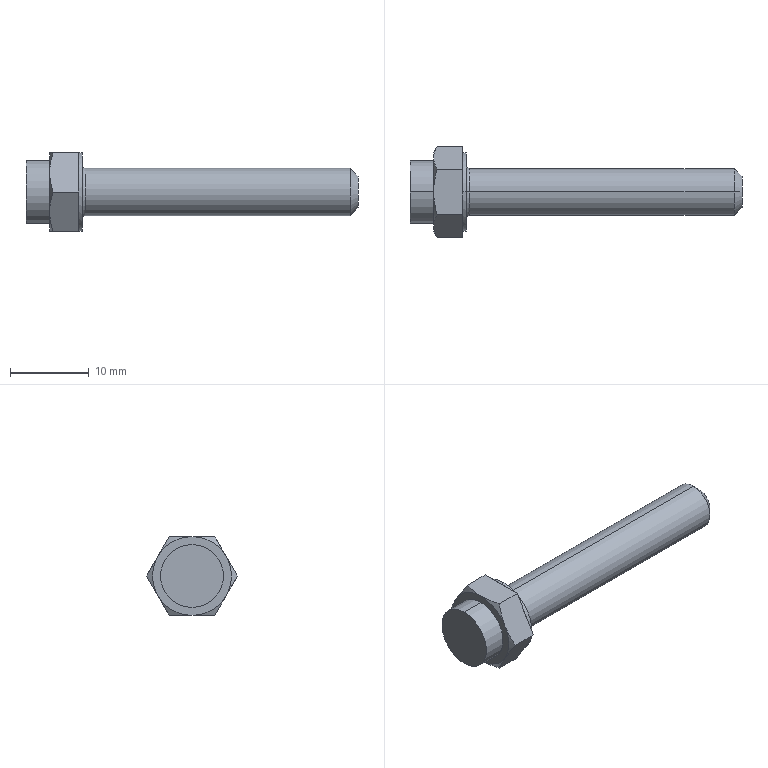Part | SolidWorks | features RevCut 4, ICE 2, Chamfer 1, Extrusion 1, Fillet 1, LPattern 1, Revolution 1 | 2 solids | 36 faces | box 42.15 x 11.547 x 10 mm | volume 1487 mm3 | plane 18 | cylinder 8 | cone 8 | torus 2 | commonest cylinder face diameters 8 x4 6 x2 10 x2
STEP:
#1=CARTESIAN_POINT('',(3.,0.,-4.));
#2=VERTEX_POINT('',#1);
#3=CARTESIAN_POINT('',(3.,0.,4.));
#4=VERTEX_POINT('',#3);
#5=CARTESIAN_POINT('',(3.,0.,0.));
#6=DIRECTION('',(-1.,0.,0.));
#7=DIRECTION('',(0.,0.,1.));
#8=AXIS2_PLACEMENT_3D('',#5,#6,#7);
#9=CIRCLE('',#8,4.);
#10=EDGE_CURVE('',#2,#4,#9,.T.);
#11=ORIENTED_EDGE('',*,*,#10,.F.);
#12=CARTESIAN_POINT('',(0.,0.,-4.));
#13=VERTEX_POINT('',#12);
#14=CARTESIAN_POINT('',(3.,0.,-4.));
#15=DIRECTION('',(-1.,0.,0.));
#16=VECTOR('',#15,1000.);
#17=LINE('',#14,#16);
#18=EDGE_CURVE('',#2,#13,#17,.T.);
#19=ORIENTED_EDGE('',*,*,#18,.T.);
#20=CARTESIAN_POINT('',(0.,0.,4.));
#21=VERTEX_POINT('',#20);
#22=CARTESIAN_POINT('',(0.,0.,0.));
#23=DIRECTION('',(-1.,0.,0.));
#24=DIRECTION('',(0.,0.,1.));
#25=AXIS2_PLACEMENT_3D('',#22,#23,#24);
#26=CIRCLE('',#25,4.);
#27=EDGE_CURVE('',#13,#21,#26,.T.);
#28=ORIENTED_EDGE('',*,*,#27,.T.);
#29=CARTESIAN_POINT('',(3.,0.,4.));
#30=DIRECTION('',(-1.,0.,0.));
#31=VECTOR('',#30,1000.);
#32=LINE('',#29,#31);
#33=EDGE_CURVE('',#4,#21,#32,.T.);
#34=ORIENTED_EDGE('',*,*,#33,.F.);
#35=EDGE_LOOP('',(#11,#19,#28,#34));
#36=FACE_OUTER_BOUND('',#35,.T.);
#37=CARTESIAN_POINT('',(3.,0.,0.));
#38=DIRECTION('',(-1.,0.,0.));
#39=DIRECTION('',(0.,0.,1.));
#40=AXIS2_PLACEMENT_3D('',#37,#38,#39);
#41=CYLINDRICAL_SURFACE('',#40,4.);
#42=ADVANCED_FACE('',(#36),#41,.F.);
#43=CARTESIAN_POINT('',(4.55,0.,3.));
#44=VERTEX_POINT('',#43);
#45=CARTESIAN_POINT('',(4.55,0.,-3.));
#46=VERTEX_POINT('',#45);
#47=CARTESIAN_POINT('',(4.55,0.,0.));
#48=DIRECTION('',(1.,0.,0.));
#49=DIRECTION('',(0.,0.,-1.));
#50=AXIS2_PLACEMENT_3D('',#47,#48,#49);
#51=CIRCLE('',#50,3.);
#52=EDGE_CURVE('',#44,#46,#51,.T.);
#53=ORIENTED_EDGE('',*,*,#52,.F.);
#54=CARTESIAN_POINT('',(4.15,0.,3.4));
#55=VERTEX_POINT('',#54);
#56=CARTESIAN_POINT('',(4.55,0.,3.4));
#57=DIRECTION('',(0.,1.,0.));
#58=DIRECTION('',(0.,0.,1.));
#59=AXIS2_PLACEMENT_3D('',#56,#57,#58);
#60=CIRCLE('',#59,0.4);
#61=EDGE_CURVE('',#44,#55,#60,.T.);
#62=ORIENTED_EDGE('',*,*,#61,.T.);
#63=CARTESIAN_POINT('',(4.15,0.,-3.4));
#64=VERTEX_POINT('',#63);
#65=CARTESIAN_POINT('',(4.15,0.,0.));
#66=DIRECTION('',(-1.,0.,0.));
#67=DIRECTION('',(0.,0.,-1.));
#68=AXIS2_PLACEMENT_3D('',#65,#66,#67);
#69=CIRCLE('',#68,3.4);
#70=EDGE_CURVE('',#64,#55,#69,.T.);
#71=ORIENTED_EDGE('',*,*,#70,.F.);
#72=CARTESIAN_POINT('',(4.55,0.,-3.4));
#73=DIRECTION('',(0.,-1.,0.));
#74=DIRECTION('',(0.,0.,-1.));
#75=AXIS2_PLACEMENT_3D('',#72,#73,#74);
#76=CIRCLE('',#75,0.4);
#77=EDGE_CURVE('',#46,#64,#76,.T.);
#78=ORIENTED_EDGE('',*,*,#77,.F.);
#79=EDGE_LOOP('',(#53,#62,#71,#78));
#80=FACE_OUTER_BOUND('',#79,.T.);
#81=CARTESIAN_POINT('',(4.55,0.,0.));
#82=DIRECTION('',(1.,0.,0.));
#83=DIRECTION('',(0.,0.,-1.));
#84=AXIS2_PLACEMENT_3D('',#81,#82,#83);
#85=TOROIDAL_SURFACE('',#84,3.4,0.4);
#86=ADVANCED_FACE('',(#80),#85,.F.);
#87=CARTESIAN_POINT('',(39.15,0.,-2.));
#88=VERTEX_POINT('',#87);
#89=CARTESIAN_POINT('',(39.15,0.,2.));
#90=VERTEX_POINT('',#89);
#91=CARTESIAN_POINT('',(39.15,0.,0.));
#92=DIRECTION('',(1.,0.,0.));
#93=DIRECTION('',(0.,0.,1.));
#94=AXIS2_PLACEMENT_3D('',#91,#92,#93);
#95=CIRCLE('',#94,2.);
#96=EDGE_CURVE('',#88,#90,#95,.T.);
#97=ORIENTED_EDGE('',*,*,#96,.F.);
#98=CARTESIAN_POINT('',(38.15,0.,-3.));
#99=VERTEX_POINT('',#98);
#100=CARTESIAN_POINT('',(38.15,0.,-3.));
#101=DIRECTION('',(-0.7071,0.,-0.7071));
#102=VECTOR('',#101,1000.);
#103=LINE('',#100,#102);
#104=EDGE_CURVE('',#88,#99,#103,.T.);
#105=ORIENTED_EDGE('',*,*,#104,.T.);
#106=CARTESIAN_POINT('',(38.15,0.,3.));
#107=VERTEX_POINT('',#106);
#108=CARTESIAN_POINT('',(38.15,0.,0.));
#109=DIRECTION('',(-1.,0.,0.));
#110=DIRECTION('',(0.,0.,1.));
#111=AXIS2_PLACEMENT_3D('',#108,#109,#110);
#112=CIRCLE('',#111,3.);
#113=EDGE_CURVE('',#107,#99,#112,.T.);
#114=ORIENTED_EDGE('',*,*,#113,.F.);
#115=CARTESIAN_POINT('',(38.15,0.,3.));
#116=DIRECTION('',(-0.7071,0.,0.7071));
#117=VECTOR('',#116,1000.);
#118=LINE('',#115,#117);
#119=EDGE_CURVE('',#90,#107,#118,.T.);
#120=ORIENTED_EDGE('',*,*,#119,.F.);
#121=EDGE_LOOP('',(#97,#105,#114,#120));
#122=FACE_OUTER_BOUND('',#121,.T.);
#123=CARTESIAN_POINT('',(38.15,0.,0.));
#124=DIRECTION('',(-1.,0.,0.));
#125=DIRECTION('',(0.,0.,1.));
#126=AXIS2_PLACEMENT_3D('',#123,#124,#125);
#127=CONICAL_SURFACE('',#126,3.,0.7854);
#128=ADVANCED_FACE('',(#122),#127,.T.);
#129=ORIENTED_EDGE('',*,*,#113,.T.);
#130=CARTESIAN_POINT('',(0.,0.,-3.));
#131=DIRECTION('',(-1.,0.,0.));
#132=VECTOR('',#131,1000.);
#133=LINE('',#130,#132);
#134=EDGE_CURVE('',#99,#46,#133,.T.);
#135=ORIENTED_EDGE('',*,*,#134,.T.);
#136=CARTESIAN_POINT('',(4.55,0.,0.));
#137=DIRECTION('',(1.,0.,0.));
#138=DIRECTION('',(0.,0.,-1.));
#139=AXIS2_PLACEMENT_3D('',#136,#137,#138);
#140=CIRCLE('',#139,3.);
#141=EDGE_CURVE('',#46,#44,#140,.T.);
#142=ORIENTED_EDGE('',*,*,#141,.T.);
#143=CARTESIAN_POINT('',(0.,0.,3.));
#144=DIRECTION('',(-1.,0.,0.));
#145=VECTOR('',#144,1000.);
#146=LINE('',#143,#145);
#147=EDGE_CURVE('',#107,#44,#146,.T.);
#148=ORIENTED_EDGE('',*,*,#147,.F.);
#149=EDGE_LOOP('',(#129,#135,#142,#148));
#150=FACE_OUTER_BOUND('',#149,.T.);
#151=CARTESIAN_POINT('',(0.,0.,0.));
#152=DIRECTION('',(-1.,0.,0.));
#153=DIRECTION('',(0.,0.,1.));
#154=AXIS2_PLACEMENT_3D('',#151,#152,#153);
#155=CYLINDRICAL_SURFACE('',#154,3.);
#156=ADVANCED_FACE('',(#150),#155,.T.);
#157=CARTESIAN_POINT('',(4.15,0.,-5.));
#158=VERTEX_POINT('',#157);
#159=CARTESIAN_POINT('',(4.15,0.,5.));
#160=VERTEX_POINT('',#159);
#161=CARTESIAN_POINT('',(4.15,0.,0.));
#162=DIRECTION('',(1.,0.,0.));
#163=DIRECTION('',(0.,0.,-1.));
#164=AXIS2_PLACEMENT_3D('',#161,#162,#163);
#165=CIRCLE('',#164,5.);
#166=EDGE_CURVE('',#158,#160,#165,.T.);
#167=ORIENTED_EDGE('',*,*,#166,.F.);
#168=CARTESIAN_POINT('',(3.65,0.,-5.));
#169=VERTEX_POINT('',#168);
#170=CARTESIAN_POINT('',(0.,0.,-5.));
#171=DIRECTION('',(-1.,0.,0.));
#172=VECTOR('',#171,1000.);
#173=LINE('',#170,#172);
#174=EDGE_CURVE('',#158,#169,#173,.T.);
#175=ORIENTED_EDGE('',*,*,#174,.T.);
#176=CARTESIAN_POINT('',(3.65,4.33,-2.5));
#177=VERTEX_POINT('',#176);
#178=CARTESIAN_POINT('',(3.65,0.,0.));
#179=DIRECTION('',(-1.,0.,0.));
#180=DIRECTION('',(0.,0.,1.));
#181=AXIS2_PLACEMENT_3D('',#178,#179,#180);
#182=CIRCLE('',#181,5.);
#183=EDGE_CURVE('',#177,#169,#182,.T.);
#184=ORIENTED_EDGE('',*,*,#183,.F.);
#185=CARTESIAN_POINT('',(3.65,4.33,2.5));
#186=VERTEX_POINT('',#185);
#187=CARTESIAN_POINT('',(3.65,0.,0.));
#188=DIRECTION('',(-1.,0.,0.));
#189=DIRECTION('',(0.,0.,1.));
#190=AXIS2_PLACEMENT_3D('',#187,#188,#189);
#191=CIRCLE('',#190,5.);
#192=EDGE_CURVE('',#186,#177,#191,.T.);
#193=ORIENTED_EDGE('',*,*,#192,.F.);
#194=CARTESIAN_POINT('',(3.65,0.,5.));
#195=VERTEX_POINT('',#194);
#196=CARTESIAN_POINT('',(3.65,0.,0.));
#197=DIRECTION('',(-1.,0.,0.));
#198=DIRECTION('',(0.,0.,1.));
#199=AXIS2_PLACEMENT_3D('',#196,#197,#198);
#200=CIRCLE('',#199,5.);
#201=EDGE_CURVE('',#195,#186,#200,.T.);
#202=ORIENTED_EDGE('',*,*,#201,.F.);
#203=CARTESIAN_POINT('',(0.,0.,5.));
#204=DIRECTION('',(-1.,0.,0.));
#205=VECTOR('',#204,1000.);
#206=LINE('',#203,#205);
#207=EDGE_CURVE('',#160,#195,#206,.T.);
#208=ORIENTED_EDGE('',*,*,#207,.F.);
#209=EDGE_LOOP('',(#167,#175,#184,#193,#202,#208));
#210=FACE_OUTER_BOUND('',#209,.T.);
#211=CARTESIAN_POINT('',(0.,0.,0.));
#212=DIRECTION('',(-1.,0.,0.));
#213=DIRECTION('',(0.,0.,1.));
#214=AXIS2_PLACEMENT_3D('',#211,#212,#213);
#215=CYLINDRICAL_SURFACE('',#214,5.);
#216=ADVANCED_FACE('',(#210),#215,.T.);
#217=CARTESIAN_POINT('',(3.65,2.887,-5.));
#218=VERTEX_POINT('',#217);
#219=CARTESIAN_POINT('',(3.65,2.887,-5.));
#220=DIRECTION('',(0.,0.5,0.866));
#221=VECTOR('',#220,1000.);
#222=LINE('',#219,#221);
#223=EDGE_CURVE('',#218,#177,#222,.T.);
#224=ORIENTED_EDGE('',*,*,#223,.F.);
#225=CARTESIAN_POINT('',(0.4466,2.887,-5.));
#226=VERTEX_POINT('',#225);
#227=CARTESIAN_POINT('',(4.15,2.887,-5.));
#228=DIRECTION('',(-1.,0.,0.));
#229=VECTOR('',#228,1000.);
#230=LINE('',#227,#229);
#231=EDGE_CURVE('',#218,#226,#230,.T.);
#232=ORIENTED_EDGE('',*,*,#231,.T.);
#233=CARTESIAN_POINT('',(0.,4.33,-2.5));
#234=VERTEX_POINT('',#233);
#235=CARTESIAN_POINT('',(0.,4.33,-2.5));
#236=CARTESIAN_POINT('',(0.,4.208,-2.712));
#237=CARTESIAN_POINT('',(0.01056,4.085,-2.925));
#238=CARTESIAN_POINT('',(0.0514,3.841,-3.347));
#239=CARTESIAN_POINT('',(0.08166,3.72,-3.556));
#240=CARTESIAN_POINT('',(0.1983,3.36,-4.181));
#241=CARTESIAN_POINT('',(0.3106,3.122,-4.592));
#242=CARTESIAN_POINT('',(0.4466,2.887,-5.));
#243=B_SPLINE_CURVE_WITH_KNOTS('',3,(#235,#236,#237,#238,#239,#240,#241,#242),.UNSPECIFIED.,.F.,.F.,(4,2,2,4),(0.002921,0.003649,0.004376,0.005831),.UNSPECIFIED.);
#244=EDGE_CURVE('',#234,#226,#243,.T.);
#245=ORIENTED_EDGE('',*,*,#244,.F.);
#246=CARTESIAN_POINT('',(0.4466,5.774,0.));
#247=VERTEX_POINT('',#246);
#248=CARTESIAN_POINT('',(0.4466,5.774,0.));
#249=CARTESIAN_POINT('',(0.1739,5.301,-0.8179));
#250=CARTESIAN_POINT('',(0.,4.822,-1.648));
#251=CARTESIAN_POINT('',(0.,4.33,-2.5));
#252=B_SPLINE_CURVE_WITH_KNOTS('',3,(#248,#249,#250,#251),.UNSPECIFIED.,.F.,.F.,(4,4),(0.000000238,0.002921),.UNSPECIFIED.);
#253=EDGE_CURVE('',#247,#234,#252,.T.);
#254=ORIENTED_EDGE('',*,*,#253,.F.);
#255=CARTESIAN_POINT('',(3.65,5.774,0.));
#256=VERTEX_POINT('',#255);
#257=CARTESIAN_POINT('',(4.15,5.774,0.));
#258=DIRECTION('',(-1.,0.,0.));
#259=VECTOR('',#258,1000.);
#260=LINE('',#257,#259);
#261=EDGE_CURVE('',#256,#247,#260,.T.);
#262=ORIENTED_EDGE('',*,*,#261,.F.);
#263=CARTESIAN_POINT('',(3.65,2.887,-5.));
#264=DIRECTION('',(0.,0.5,0.866));
#265=VECTOR('',#264,1000.);
#266=LINE('',#263,#265);
#267=EDGE_CURVE('',#177,#256,#266,.T.);
#268=ORIENTED_EDGE('',*,*,#267,.F.);
#269=EDGE_LOOP('',(#224,#232,#245,#254,#262,#268));
#270=FACE_OUTER_BOUND('',#269,.T.);
#271=CARTESIAN_POINT('',(4.15,2.887,-5.));
#272=DIRECTION('',(0.,-0.866,0.5));
#273=DIRECTION('',(0.,-0.5,-0.866));
#274=AXIS2_PLACEMENT_3D('',#271,#272,#273);
#275=PLANE('',#274);
#276=ADVANCED_FACE('',(#270),#275,.F.);
#277=CARTESIAN_POINT('',(3.65,5.774,0.));
#278=DIRECTION('',(0.,-0.5,0.866));
#279=VECTOR('',#278,1000.);
#280=LINE('',#277,#279);
#281=EDGE_CURVE('',#256,#186,#280,.T.);
#282=ORIENTED_EDGE('',*,*,#281,.F.);
#283=ORIENTED_EDGE('',*,*,#261,.T.);
#284=CARTESIAN_POINT('',(0.,4.33,2.5));
#285=VERTEX_POINT('',#284);
#286=CARTESIAN_POINT('',(0.,4.33,2.5));
#287=CARTESIAN_POINT('',(0.,4.453,2.288));
#288=CARTESIAN_POINT('',(0.01056,4.576,2.075));
#289=CARTESIAN_POINT('',(0.0514,4.819,1.653));
#290=CARTESIAN_POINT('',(0.08166,4.94,1.444));
#291=CARTESIAN_POINT('',(0.1983,5.3,0.8193));
#292=CARTESIAN_POINT('',(0.3106,5.538,0.4079));
#293=CARTESIAN_POINT('',(0.4466,5.774,0.));
#294=B_SPLINE_CURVE_WITH_KNOTS('',3,(#286,#287,#288,#289,#290,#291,#292,#293),.UNSPECIFIED.,.F.,.F.,(4,2,2,4),(0.002921,0.003649,0.004376,0.005831),.UNSPECIFIED.);
#295=EDGE_CURVE('',#285,#247,#294,.T.);
#296=ORIENTED_EDGE('',*,*,#295,.F.);
#297=CARTESIAN_POINT('',(0.4466,2.887,5.));
#298=VERTEX_POINT('',#297);
#299=CARTESIAN_POINT('',(0.4466,2.887,5.));
#300=CARTESIAN_POINT('',(0.1739,3.359,4.182));
#301=CARTESIAN_POINT('',(0.,3.838,3.352));
#302=CARTESIAN_POINT('',(0.,4.33,2.5));
#303=B_SPLINE_CURVE_WITH_KNOTS('',3,(#299,#300,#301,#302),.UNSPECIFIED.,.F.,.F.,(4,4),(0.000000238,0.002921),.UNSPECIFIED.);
#304=EDGE_CURVE('',#298,#285,#303,.T.);
#305=ORIENTED_EDGE('',*,*,#304,.F.);
#306=CARTESIAN_POINT('',(3.65,2.887,5.));
#307=VERTEX_POINT('',#306);
#308=CARTESIAN_POINT('',(4.15,2.887,5.));
#309=DIRECTION('',(-1.,0.,0.));
#310=VECTOR('',#309,1000.);
#311=LINE('',#308,#310);
#312=EDGE_CURVE('',#307,#298,#311,.T.);
#313=ORIENTED_EDGE('',*,*,#312,.F.);
#314=CARTESIAN_POINT('',(3.65,5.774,0.));
#315=DIRECTION('',(0.,-0.5,0.866));
#316=VECTOR('',#315,1000.);
#317=LINE('',#314,#316);
#318=EDGE_CURVE('',#186,#307,#317,.T.);
#319=ORIENTED_EDGE('',*,*,#318,.F.);
#320=EDGE_LOOP('',(#282,#283,#296,#305,#313,#319));
#321=FACE_OUTER_BOUND('',#320,.T.);
#322=CARTESIAN_POINT('',(4.15,5.774,0.));
#323=DIRECTION('',(0.,-0.866,-0.5));
#324=DIRECTION('',(0.,0.5,-0.866));
#325=AXIS2_PLACEMENT_3D('',#322,#323,#324);
#326=PLANE('',#325);
#327=ADVANCED_FACE('',(#321),#326,.F.);
#328=CARTESIAN_POINT('',(3.65,2.887,5.));
#329=DIRECTION('',(0.,-1.,0.));
#330=VECTOR('',#329,1000.);
#331=LINE('',#328,#330);
#332=EDGE_CURVE('',#307,#195,#331,.T.);
#333=ORIENTED_EDGE('',*,*,#332,.F.);
#334=ORIENTED_EDGE('',*,*,#312,.T.);
#335=CARTESIAN_POINT('',(0.,0.,5.));
#336=VERTEX_POINT('',#335);
#337=CARTESIAN_POINT('',(0.,0.,5.));
#338=CARTESIAN_POINT('',(0.,0.4887,5.));
#339=CARTESIAN_POINT('',(0.04321,0.9837,5.));
#340=CARTESIAN_POINT('',(0.1996,1.947,5.));
#341=CARTESIAN_POINT('',(0.3118,2.42,5.));
#342=CARTESIAN_POINT('',(0.4466,2.887,5.));
#343=B_SPLINE_CURVE_WITH_KNOTS('',3,(#337,#338,#339,#340,#341,#342),.UNSPECIFIED.,.F.,.F.,(4,2,4),(0.008262,0.009724,0.01119),.UNSPECIFIED.);
#344=EDGE_CURVE('',#336,#298,#343,.T.);
#345=ORIENTED_EDGE('',*,*,#344,.F.);
#346=CARTESIAN_POINT('',(0.4466,-2.887,5.));
#347=VERTEX_POINT('',#346);
#348=CARTESIAN_POINT('',(0.4466,-2.887,5.));
#349=CARTESIAN_POINT('',(0.3109,-2.417,5.));
#350=CARTESIAN_POINT('',(0.1973,-1.936,5.));
#351=CARTESIAN_POINT('',(0.04202,-0.9731,5.));
#352=CARTESIAN_POINT('',(0.,-0.4884,5.));
#353=CARTESIAN_POINT('',(0.,0.,5.));
#354=B_SPLINE_CURVE_WITH_KNOTS('',3,(#348,#349,#350,#351,#352,#353),.UNSPECIFIED.,.F.,.F.,(4,2,4),(0.00534,0.006801,0.008262),.UNSPECIFIED.);
#355=EDGE_CURVE('',#347,#336,#354,.T.);
#356=ORIENTED_EDGE('',*,*,#355,.F.);
#357=CARTESIAN_POINT('',(3.65,-2.887,5.));
#358=VERTEX_POINT('',#357);
#359=CARTESIAN_POINT('',(4.15,-2.887,5.));
#360=DIRECTION('',(-1.,0.,0.));
#361=VECTOR('',#360,1000.);
#362=LINE('',#359,#361);
#363=EDGE_CURVE('',#358,#347,#362,.T.);
#364=ORIENTED_EDGE('',*,*,#363,.F.);
#365=CARTESIAN_POINT('',(3.65,2.887,5.));
#366=DIRECTION('',(0.,-1.,0.));
#367=VECTOR('',#366,1000.);
#368=LINE('',#365,#367);
#369=EDGE_CURVE('',#195,#358,#368,.T.);
#370=ORIENTED_EDGE('',*,*,#369,.F.);
#371=EDGE_LOOP('',(#333,#334,#345,#356,#364,#370));
#372=FACE_OUTER_BOUND('',#371,.T.);
#373=CARTESIAN_POINT('',(4.15,2.887,5.));
#374=DIRECTION('',(0.,0.,-1.));
#375=DIRECTION('',(-1.,0.,0.));
#376=AXIS2_PLACEMENT_3D('',#373,#374,#375);
#377=PLANE('',#376);
#378=ADVANCED_FACE('',(#372),#377,.F.);
#379=CARTESIAN_POINT('',(3.65,-4.33,2.5));
#380=VERTEX_POINT('',#379);
#381=CARTESIAN_POINT('',(3.65,-5.774,0.));
#382=DIRECTION('',(0.,-0.5,-0.866));
#383=VECTOR('',#382,1000.);
#384=LINE('',#381,#383);
#385=EDGE_CURVE('',#358,#380,#384,.T.);
#386=ORIENTED_EDGE('',*,*,#385,.F.);
#387=ORIENTED_EDGE('',*,*,#363,.T.);
#388=CARTESIAN_POINT('',(0.,-4.33,2.5));
#389=VERTEX_POINT('',#388);
#390=CARTESIAN_POINT('',(0.,-4.33,2.5));
#391=CARTESIAN_POINT('',(0.,-4.208,2.712));
#392=CARTESIAN_POINT('',(0.01056,-4.085,2.925));
#393=CARTESIAN_POINT('',(0.0514,-3.841,3.347));
#394=CARTESIAN_POINT('',(0.08166,-3.72,3.556));
#395=CARTESIAN_POINT('',(0.1983,-3.36,4.181));
#396=CARTESIAN_POINT('',(0.3106,-3.122,4.592));
#397=CARTESIAN_POINT('',(0.4466,-2.887,5.));
#398=B_SPLINE_CURVE_WITH_KNOTS('',3,(#390,#391,#392,#393,#394,#395,#396,#397),.UNSPECIFIED.,.F.,.F.,(4,2,2,4),(0.002921,0.003649,0.004376,0.005831),.UNSPECIFIED.);
#399=EDGE_CURVE('',#389,#347,#398,.T.);
#400=ORIENTED_EDGE('',*,*,#399,.F.);
#401=CARTESIAN_POINT('',(0.4466,-5.774,0.));
#402=VERTEX_POINT('',#401);
#403=CARTESIAN_POINT('',(0.4466,-5.774,0.));
#404=CARTESIAN_POINT('',(0.1739,-5.301,0.8179));
#405=CARTESIAN_POINT('',(0.,-4.822,1.648));
#406=CARTESIAN_POINT('',(0.,-4.33,2.5));
#407=B_SPLINE_CURVE_WITH_KNOTS('',3,(#403,#404,#405,#406),.UNSPECIFIED.,.F.,.F.,(4,4),(0.000000238,0.002921),.UNSPECIFIED.);
#408=EDGE_CURVE('',#402,#389,#407,.T.);
#409=ORIENTED_EDGE('',*,*,#408,.F.);
#410=CARTESIAN_POINT('',(3.65,-5.774,0.));
#411=VERTEX_POINT('',#410);
#412=CARTESIAN_POINT('',(4.15,-5.774,0.));
#413=DIRECTION('',(-1.,0.,0.));
#414=VECTOR('',#413,1000.);
#415=LINE('',#412,#414);
#416=EDGE_CURVE('',#411,#402,#415,.T.);
#417=ORIENTED_EDGE('',*,*,#416,.F.);
#418=CARTESIAN_POINT('',(3.65,-5.774,0.));
#419=DIRECTION('',(0.,-0.5,-0.866));
#420=VECTOR('',#419,1000.);
#421=LINE('',#418,#420);
#422=EDGE_CURVE('',#380,#411,#421,.T.);
#423=ORIENTED_EDGE('',*,*,#422,.F.);
#424=EDGE_LOOP('',(#386,#387,#400,#409,#417,#423));
#425=FACE_OUTER_BOUND('',#424,.T.);
#426=CARTESIAN_POINT('',(4.15,-5.774,0.));
#427=DIRECTION('',(0.,0.866,-0.5));
#428=DIRECTION('',(0.,0.5,0.866));
#429=AXIS2_PLACEMENT_3D('',#426,#427,#428);
#430=PLANE('',#429);
#431=ADVANCED_FACE('',(#425),#430,.F.);
#432=CARTESIAN_POINT('',(3.65,-4.33,-2.5));
#433=VERTEX_POINT('',#432);
#434=CARTESIAN_POINT('',(3.65,-2.887,-5.));
#435=DIRECTION('',(0.,0.5,-0.866));
#436=VECTOR('',#435,1000.);
#437=LINE('',#434,#436);
#438=EDGE_CURVE('',#411,#433,#437,.T.);
#439=ORIENTED_EDGE('',*,*,#438,.F.);
#440=ORIENTED_EDGE('',*,*,#416,.T.);
#441=CARTESIAN_POINT('',(0.,-4.33,-2.5));
#442=VERTEX_POINT('',#441);
#443=CARTESIAN_POINT('',(0.,-4.33,-2.5));
#444=CARTESIAN_POINT('',(0.,-4.453,-2.288));
#445=CARTESIAN_POINT('',(0.01056,-4.576,-2.075));
#446=CARTESIAN_POINT('',(0.0514,-4.819,-1.653));
#447=CARTESIAN_POINT('',(0.08166,-4.94,-1.444));
#448=CARTESIAN_POINT('',(0.1983,-5.3,-0.8193));
#449=CARTESIAN_POINT('',(0.3106,-5.538,-0.4079));
#450=CARTESIAN_POINT('',(0.4466,-5.774,0.));
#451=B_SPLINE_CURVE_WITH_KNOTS('',3,(#443,#444,#445,#446,#447,#448,#449,#450),.UNSPECIFIED.,.F.,.F.,(4,2,2,4),(0.002921,0.003649,0.004376,0.005831),.UNSPECIFIED.);
#452=EDGE_CURVE('',#442,#402,#451,.T.);
#453=ORIENTED_EDGE('',*,*,#452,.F.);
#454=CARTESIAN_POINT('',(0.4466,-2.887,-5.));
#455=VERTEX_POINT('',#454);
#456=CARTESIAN_POINT('',(0.4466,-2.887,-5.));
#457=CARTESIAN_POINT('',(0.1739,-3.359,-4.182));
#458=CARTESIAN_POINT('',(0.,-3.838,-3.352));
#459=CARTESIAN_POINT('',(0.,-4.33,-2.5));
#460=B_SPLINE_CURVE_WITH_KNOTS('',3,(#456,#457,#458,#459),.UNSPECIFIED.,.F.,.F.,(4,4),(0.000000238,0.002921),.UNSPECIFIED.);
#461=EDGE_CURVE('',#455,#442,#460,.T.);
#462=ORIENTED_EDGE('',*,*,#461,.F.);
#463=CARTESIAN_POINT('',(3.65,-2.887,-5.));
#464=VERTEX_POINT('',#463);
#465=CARTESIAN_POINT('',(4.15,-2.887,-5.));
#466=DIRECTION('',(-1.,0.,0.));
#467=VECTOR('',#466,1000.);
#468=LINE('',#465,#467);
#469=EDGE_CURVE('',#464,#455,#468,.T.);
#470=ORIENTED_EDGE('',*,*,#469,.F.);
#471=CARTESIAN_POINT('',(3.65,-2.887,-5.));
#472=DIRECTION('',(0.,0.5,-0.866));
#473=VECTOR('',#472,1000.);
#474=LINE('',#471,#473);
#475=EDGE_CURVE('',#433,#464,#474,.T.);
#476=ORIENTED_EDGE('',*,*,#475,.F.);
#477=EDGE_LOOP('',(#439,#440,#453,#462,#470,#476));
#478=FACE_OUTER_BOUND('',#477,.T.);
#479=CARTESIAN_POINT('',(4.15,-2.887,-5.));
#480=DIRECTION('',(0.,0.866,0.5));
#481=DIRECTION('',(0.,-0.5,0.866));
#482=AXIS2_PLACEMENT_3D('',#479,#480,#481);
#483=PLANE('',#482);
#484=ADVANCED_FACE('',(#478),#483,.F.);
#485=CARTESIAN_POINT('',(3.65,2.887,-5.));
#486=DIRECTION('',(0.,1.,0.));
#487=VECTOR('',#486,1000.);
#488=LINE('',#485,#487);
#489=EDGE_CURVE('',#464,#169,#488,.T.);
#490=ORIENTED_EDGE('',*,*,#489,.F.);
#491=ORIENTED_EDGE('',*,*,#469,.T.);
#492=CARTESIAN_POINT('',(0.,0.,-5.));
#493=VERTEX_POINT('',#492);
#494=CARTESIAN_POINT('',(0.,0.,-5.));
#495=CARTESIAN_POINT('',(0.,-0.4884,-5.));
#496=CARTESIAN_POINT('',(0.04202,-0.9731,-5.));
#497=CARTESIAN_POINT('',(0.1973,-1.936,-5.));
#498=CARTESIAN_POINT('',(0.3109,-2.417,-5.));
#499=CARTESIAN_POINT('',(0.4466,-2.887,-5.));
#500=B_SPLINE_CURVE_WITH_KNOTS('',3,(#494,#495,#496,#497,#498,#499),.UNSPECIFIED.,.F.,.F.,(4,2,4),(0.01799,0.01945,0.02091),.UNSPECIFIED.);
#501=EDGE_CURVE('',#493,#455,#500,.T.);
#502=ORIENTED_EDGE('',*,*,#501,.F.);
#503=CARTESIAN_POINT('',(0.4466,2.887,-5.));
#504=CARTESIAN_POINT('',(0.3118,2.42,-5.));
#505=CARTESIAN_POINT('',(0.1996,1.947,-5.));
#506=CARTESIAN_POINT('',(0.04321,0.9837,-5.));
#507=CARTESIAN_POINT('',(0.,0.4887,-5.));
#508=CARTESIAN_POINT('',(0.,0.,-5.));
#509=B_SPLINE_CURVE_WITH_KNOTS('',3,(#503,#504,#505,#506,#507,#508),.UNSPECIFIED.,.F.,.F.,(4,2,4),(0.01507,0.01653,0.01799),.UNSPECIFIED.);
#510=EDGE_CURVE('',#226,#493,#509,.T.);
#511=ORIENTED_EDGE('',*,*,#510,.F.);
#512=ORIENTED_EDGE('',*,*,#231,.F.);
#513=CARTESIAN_POINT('',(3.65,2.887,-5.));
#514=DIRECTION('',(0.,1.,0.));
#515=VECTOR('',#514,1000.);
#516=LINE('',#513,#515);
#517=EDGE_CURVE('',#169,#218,#516,.T.);
#518=ORIENTED_EDGE('',*,*,#517,.F.);
#519=EDGE_LOOP('',(#490,#491,#502,#511,#512,#518));
#520=FACE_OUTER_BOUND('',#519,.T.);
#521=CARTESIAN_POINT('',(4.15,2.887,-5.));
#522=DIRECTION('',(0.,0.,1.));
#523=DIRECTION('',(1.,0.,0.));
#524=AXIS2_PLACEMENT_3D('',#521,#522,#523);
#525=PLANE('',#524);
#526=ADVANCED_FACE('',(#520),#525,.F.);
#527=ORIENTED_EDGE('',*,*,#461,.T.);
#528=CARTESIAN_POINT('',(0.,0.,0.));
#529=DIRECTION('',(1.,0.,0.));
#530=DIRECTION('',(0.,0.,-1.));
#531=AXIS2_PLACEMENT_3D('',#528,#529,#530);
#532=CIRCLE('',#531,5.);
#533=EDGE_CURVE('',#442,#493,#532,.T.);
#534=ORIENTED_EDGE('',*,*,#533,.T.);
#535=ORIENTED_EDGE('',*,*,#501,.T.);
#536=EDGE_LOOP('',(#527,#534,#535));
#537=FACE_OUTER_BOUND('',#536,.T.);
#538=CARTESIAN_POINT('',(0.,0.,0.));
#539=DIRECTION('',(1.,0.,0.));
#540=DIRECTION('',(0.,0.,-1.));
#541=AXIS2_PLACEMENT_3D('',#538,#539,#540);
#542=CONICAL_SURFACE('',#541,5.,1.047);
#543=ADVANCED_FACE('',(#537),#542,.T.);
#544=ORIENTED_EDGE('',*,*,#408,.T.);
#545=CARTESIAN_POINT('',(0.,0.,0.));
#546=DIRECTION('',(1.,0.,0.));
#547=DIRECTION('',(0.,0.,-1.));
#548=AXIS2_PLACEMENT_3D('',#545,#546,#547);
#549=CIRCLE('',#548,5.);
#550=EDGE_CURVE('',#389,#442,#549,.T.);
#551=ORIENTED_EDGE('',*,*,#550,.T.);
#552=ORIENTED_EDGE('',*,*,#452,.T.);
#553=EDGE_LOOP('',(#544,#551,#552));
#554=FACE_OUTER_BOUND('',#553,.T.);
#555=CARTESIAN_POINT('',(0.,0.,0.));
#556=DIRECTION('',(1.,0.,0.));
#557=DIRECTION('',(0.,0.,-1.));
#558=AXIS2_PLACEMENT_3D('',#555,#556,#557);
#559=CONICAL_SURFACE('',#558,5.,1.047);
#560=ADVANCED_FACE('',(#554),#559,.T.);
#561=ORIENTED_EDGE('',*,*,#355,.T.);
#562=CARTESIAN_POINT('',(0.,0.,0.));
#563=DIRECTION('',(1.,0.,0.));
#564=DIRECTION('',(0.,0.,-1.));
#565=AXIS2_PLACEMENT_3D('',#562,#563,#564);
#566=CIRCLE('',#565,5.);
#567=EDGE_CURVE('',#336,#389,#566,.T.);
#568=ORIENTED_EDGE('',*,*,#567,.T.);
#569=ORIENTED_EDGE('',*,*,#399,.T.);
#570=EDGE_LOOP('',(#561,#568,#569));
#571=FACE_OUTER_BOUND('',#570,.T.);
#572=CARTESIAN_POINT('',(0.,0.,0.));
#573=DIRECTION('',(1.,0.,0.));
#574=DIRECTION('',(0.,0.,-1.));
#575=AXIS2_PLACEMENT_3D('',#572,#573,#574);
#576=CONICAL_SURFACE('',#575,5.,1.047);
#577=ADVANCED_FACE('',(#571),#576,.T.);
#578=ORIENTED_EDGE('',*,*,#344,.T.);
#579=ORIENTED_EDGE('',*,*,#304,.T.);
#580=CARTESIAN_POINT('',(0.,0.,0.));
#581=DIRECTION('',(-1.,0.,0.));
#582=DIRECTION('',(0.,0.,1.));
#583=AXIS2_PLACEMENT_3D('',#580,#581,#582);
#584=CIRCLE('',#583,5.);
#585=EDGE_CURVE('',#336,#285,#584,.T.);
#586=ORIENTED_EDGE('',*,*,#585,.F.);
#587=EDGE_LOOP('',(#578,#579,#586));
#588=FACE_OUTER_BOUND('',#587,.T.);
#589=CARTESIAN_POINT('',(0.,0.,0.));
#590=DIRECTION('',(1.,0.,0.));
#591=DIRECTION('',(0.,0.,-1.));
#592=AXIS2_PLACEMENT_3D('',#589,#590,#591);
#593=CONICAL_SURFACE('',#592,5.,1.047);
#594=ADVANCED_FACE('',(#588),#593,.T.);
#595=ORIENTED_EDGE('',*,*,#295,.T.);
#596=ORIENTED_EDGE('',*,*,#253,.T.);
#597=CARTESIAN_POINT('',(0.,0.,0.));
#598=DIRECTION('',(1.,0.,0.));
#599=DIRECTION('',(0.,0.,-1.));
#600=AXIS2_PLACEMENT_3D('',#597,#598,#599);
#601=CIRCLE('',#600,5.);
#602=EDGE_CURVE('',#234,#285,#601,.T.);
#603=ORIENTED_EDGE('',*,*,#602,.T.);
#604=EDGE_LOOP('',(#595,#596,#603));
#605=FACE_OUTER_BOUND('',#604,.T.);
#606=CARTESIAN_POINT('',(0.,0.,0.));
#607=DIRECTION('',(1.,0.,0.));
#608=DIRECTION('',(0.,0.,-1.));
#609=AXIS2_PLACEMENT_3D('',#606,#607,#608);
#610=CONICAL_SURFACE('',#609,5.,1.047);
#611=ADVANCED_FACE('',(#605),#610,.T.);
#612=ORIENTED_EDGE('',*,*,#244,.T.);
#613=ORIENTED_EDGE('',*,*,#510,.T.);
#614=CARTESIAN_POINT('',(0.,0.,0.));
#615=DIRECTION('',(1.,0.,0.));
#616=DIRECTION('',(0.,0.,-1.));
#617=AXIS2_PLACEMENT_3D('',#614,#615,#616);
#618=CIRCLE('',#617,5.);
#619=EDGE_CURVE('',#493,#234,#618,.T.);
#620=ORIENTED_EDGE('',*,*,#619,.T.);
#621=EDGE_LOOP('',(#612,#613,#620));
#622=FACE_OUTER_BOUND('',#621,.T.);
#623=CARTESIAN_POINT('',(0.,0.,0.));
#624=DIRECTION('',(1.,0.,0.));
#625=DIRECTION('',(0.,0.,-1.));
#626=AXIS2_PLACEMENT_3D('',#623,#624,#625);
#627=CONICAL_SURFACE('',#626,5.,1.047);
#628=ADVANCED_FACE('',(#622),#627,.T.);
#629=CARTESIAN_POINT('',(0.,0.,0.));
#630=DIRECTION('',(-1.,0.,0.));
#631=DIRECTION('',(0.,0.,1.));
#632=AXIS2_PLACEMENT_3D('',#629,#630,#631);
#633=CIRCLE('',#632,4.);
#634=EDGE_CURVE('',#21,#13,#633,.T.);
#635=ORIENTED_EDGE('',*,*,#634,.F.);
#636=ORIENTED_EDGE('',*,*,#27,.F.);
#637=EDGE_LOOP('',(#635,#636));
#638=FACE_BOUND('',#637,.T.);
#639=ORIENTED_EDGE('',*,*,#619,.F.);
#640=ORIENTED_EDGE('',*,*,#533,.F.);
#641=ORIENTED_EDGE('',*,*,#550,.F.);
#642=ORIENTED_EDGE('',*,*,#567,.F.);
#643=ORIENTED_EDGE('',*,*,#585,.T.);
#644=ORIENTED_EDGE('',*,*,#602,.F.);
#645=EDGE_LOOP('',(#639,#640,#641,#642,#643,#644));
#646=FACE_OUTER_BOUND('',#645,.T.);
#647=CARTESIAN_POINT('',(0.,5.774,0.));
#648=DIRECTION('',(1.,0.,0.));
#649=DIRECTION('',(0.,0.,-1.));
#650=AXIS2_PLACEMENT_3D('',#647,#648,#649);
#651=PLANE('',#650);
#652=ADVANCED_FACE('',(#638,#646),#651,.F.);
#653=ORIENTED_EDGE('',*,*,#223,.T.);
#654=ORIENTED_EDGE('',*,*,#183,.T.);
#655=ORIENTED_EDGE('',*,*,#517,.T.);
#656=EDGE_LOOP('',(#653,#654,#655));
#657=FACE_OUTER_BOUND('',#656,.T.);
#658=CARTESIAN_POINT('',(3.65,5.,0.));
#659=DIRECTION('',(1.,0.,0.));
#660=DIRECTION('',(0.,0.,-1.));
#661=AXIS2_PLACEMENT_3D('',#658,#659,#660);
#662=PLANE('',#661);
#663=ADVANCED_FACE('',(#657),#662,.T.);
#664=ORIENTED_EDGE('',*,*,#267,.T.);
#665=ORIENTED_EDGE('',*,*,#281,.T.);
#666=ORIENTED_EDGE('',*,*,#192,.T.);
#667=EDGE_LOOP('',(#664,#665,#666));
#668=FACE_OUTER_BOUND('',#667,.T.);
#669=CARTESIAN_POINT('',(3.65,5.,0.));
#670=DIRECTION('',(1.,0.,0.));
#671=DIRECTION('',(0.,0.,-1.));
#672=AXIS2_PLACEMENT_3D('',#669,#670,#671);
#673=PLANE('',#672);
#674=ADVANCED_FACE('',(#668),#673,.T.);
#675=ORIENTED_EDGE('',*,*,#318,.T.);
#676=ORIENTED_EDGE('',*,*,#332,.T.);
#677=ORIENTED_EDGE('',*,*,#201,.T.);
#678=EDGE_LOOP('',(#675,#676,#677));
#679=FACE_OUTER_BOUND('',#678,.T.);
#680=CARTESIAN_POINT('',(3.65,5.,0.));
#681=DIRECTION('',(1.,0.,0.));
#682=DIRECTION('',(0.,0.,-1.));
#683=AXIS2_PLACEMENT_3D('',#680,#681,#682);
#684=PLANE('',#683);
#685=ADVANCED_FACE('',(#679),#684,.T.);
#686=ORIENTED_EDGE('',*,*,#369,.T.);
#687=ORIENTED_EDGE('',*,*,#385,.T.);
#688=CARTESIAN_POINT('',(3.65,0.,0.));
#689=DIRECTION('',(-1.,0.,0.));
#690=DIRECTION('',(0.,0.,1.));
#691=AXIS2_PLACEMENT_3D('',#688,#689,#690);
#692=CIRCLE('',#691,5.);
#693=EDGE_CURVE('',#380,#195,#692,.T.);
#694=ORIENTED_EDGE('',*,*,#693,.T.);
#695=EDGE_LOOP('',(#686,#687,#694));
#696=FACE_OUTER_BOUND('',#695,.T.);
#697=CARTESIAN_POINT('',(3.65,5.,0.));
#698=DIRECTION('',(1.,0.,0.));
#699=DIRECTION('',(0.,0.,-1.));
#700=AXIS2_PLACEMENT_3D('',#697,#698,#699);
#701=PLANE('',#700);
#702=ADVANCED_FACE('',(#696),#701,.T.);
#703=ORIENTED_EDGE('',*,*,#422,.T.);
#704=ORIENTED_EDGE('',*,*,#438,.T.);
#705=CARTESIAN_POINT('',(3.65,0.,0.));
#706=DIRECTION('',(-1.,0.,0.));
#707=DIRECTION('',(0.,0.,1.));
#708=AXIS2_PLACEMENT_3D('',#705,#706,#707);
#709=CIRCLE('',#708,5.);
#710=EDGE_CURVE('',#433,#380,#709,.T.);
#711=ORIENTED_EDGE('',*,*,#710,.T.);
#712=EDGE_LOOP('',(#703,#704,#711));
#713=FACE_OUTER_BOUND('',#712,.T.);
#714=CARTESIAN_POINT('',(3.65,5.,0.));
#715=DIRECTION('',(1.,0.,0.));
#716=DIRECTION('',(0.,0.,-1.));
#717=AXIS2_PLACEMENT_3D('',#714,#715,#716);
#718=PLANE('',#717);
#719=ADVANCED_FACE('',(#713),#718,.T.);
#720=ORIENTED_EDGE('',*,*,#475,.T.);
#721=ORIENTED_EDGE('',*,*,#489,.T.);
#722=CARTESIAN_POINT('',(3.65,0.,0.));
#723=DIRECTION('',(-1.,0.,0.));
#724=DIRECTION('',(0.,0.,1.));
#725=AXIS2_PLACEMENT_3D('',#722,#723,#724);
#726=CIRCLE('',#725,5.);
#727=EDGE_CURVE('',#169,#433,#726,.T.);
#728=ORIENTED_EDGE('',*,*,#727,.T.);
#729=EDGE_LOOP('',(#720,#721,#728));
#730=FACE_OUTER_BOUND('',#729,.T.);
#731=CARTESIAN_POINT('',(3.65,5.,0.));
#732=DIRECTION('',(1.,0.,0.));
#733=DIRECTION('',(0.,0.,-1.));
#734=AXIS2_PLACEMENT_3D('',#731,#732,#733);
#735=PLANE('',#734);
#736=ADVANCED_FACE('',(#730),#735,.T.);
#737=ORIENTED_EDGE('',*,*,#174,.F.);
#738=CARTESIAN_POINT('',(4.15,0.,0.));
#739=DIRECTION('',(1.,0.,0.));
#740=DIRECTION('',(0.,0.,-1.));
#741=AXIS2_PLACEMENT_3D('',#738,#739,#740);
#742=CIRCLE('',#741,5.);
#743=EDGE_CURVE('',#160,#158,#742,.T.);
#744=ORIENTED_EDGE('',*,*,#743,.F.);
#745=ORIENTED_EDGE('',*,*,#207,.T.);
#746=ORIENTED_EDGE('',*,*,#693,.F.);
#747=ORIENTED_EDGE('',*,*,#710,.F.);
#748=ORIENTED_EDGE('',*,*,#727,.F.);
#749=EDGE_LOOP('',(#737,#744,#745,#746,#747,#748));
#750=FACE_OUTER_BOUND('',#749,.T.);
#751=CARTESIAN_POINT('',(0.,0.,0.));
#752=DIRECTION('',(-1.,0.,0.));
#753=DIRECTION('',(0.,0.,1.));
#754=AXIS2_PLACEMENT_3D('',#751,#752,#753);
#755=CYLINDRICAL_SURFACE('',#754,5.);
#756=ADVANCED_FACE('',(#750),#755,.T.);
#757=CARTESIAN_POINT('',(39.15,0.,0.));
#758=DIRECTION('',(1.,0.,0.));
#759=DIRECTION('',(0.,0.,1.));
#760=AXIS2_PLACEMENT_3D('',#757,#758,#759);
#761=CIRCLE('',#760,2.);
#762=EDGE_CURVE('',#90,#88,#761,.T.);
#763=ORIENTED_EDGE('',*,*,#762,.T.);
#764=ORIENTED_EDGE('',*,*,#96,.T.);
#765=EDGE_LOOP('',(#763,#764));
#766=FACE_OUTER_BOUND('',#765,.T.);
#767=CARTESIAN_POINT('',(39.15,0.,0.));
#768=DIRECTION('',(-1.,0.,0.));
#769=DIRECTION('',(0.,0.,1.));
#770=AXIS2_PLACEMENT_3D('',#767,#768,#769);
#771=PLANE('',#770);
#772=ADVANCED_FACE('',(#766),#771,.F.);
#773=ORIENTED_EDGE('',*,*,#134,.F.);
#774=CARTESIAN_POINT('',(38.15,0.,0.));
#775=DIRECTION('',(-1.,0.,0.));
#776=DIRECTION('',(0.,0.,1.));
#777=AXIS2_PLACEMENT_3D('',#774,#775,#776);
#778=CIRCLE('',#777,3.);
#779=EDGE_CURVE('',#99,#107,#778,.T.);
#780=ORIENTED_EDGE('',*,*,#779,.T.);
#781=ORIENTED_EDGE('',*,*,#147,.T.);
#782=ORIENTED_EDGE('',*,*,#52,.T.);
#783=EDGE_LOOP('',(#773,#780,#781,#782));
#784=FACE_OUTER_BOUND('',#783,.T.);
#785=CARTESIAN_POINT('',(0.,0.,0.));
#786=DIRECTION('',(-1.,0.,0.));
#787=DIRECTION('',(0.,0.,1.));
#788=AXIS2_PLACEMENT_3D('',#785,#786,#787);
#789=CYLINDRICAL_SURFACE('',#788,3.);
#790=ADVANCED_FACE('',(#784),#789,.T.);
#791=ORIENTED_EDGE('',*,*,#70,.T.);
#792=CARTESIAN_POINT('',(4.15,0.,0.));
#793=DIRECTION('',(-1.,0.,0.));
#794=DIRECTION('',(0.,0.,-1.));
#795=AXIS2_PLACEMENT_3D('',#792,#793,#794);
#796=CIRCLE('',#795,3.4);
#797=EDGE_CURVE('',#55,#64,#796,.T.);
#798=ORIENTED_EDGE('',*,*,#797,.T.);
#799=EDGE_LOOP('',(#791,#798));
#800=FACE_BOUND('',#799,.T.);
#801=ORIENTED_EDGE('',*,*,#743,.T.);
#802=ORIENTED_EDGE('',*,*,#166,.T.);
#803=EDGE_LOOP('',(#801,#802));
#804=FACE_OUTER_BOUND('',#803,.T.);
#805=CARTESIAN_POINT('',(4.15,5.774,0.));
#806=DIRECTION('',(1.,0.,0.));
#807=DIRECTION('',(0.,0.,-1.));
#808=AXIS2_PLACEMENT_3D('',#805,#806,#807);
#809=PLANE('',#808);
#810=ADVANCED_FACE('',(#800,#804),#809,.T.);
#811=ORIENTED_EDGE('',*,*,#104,.F.);
#812=ORIENTED_EDGE('',*,*,#762,.F.);
#813=ORIENTED_EDGE('',*,*,#119,.T.);
#814=ORIENTED_EDGE('',*,*,#779,.F.);
#815=EDGE_LOOP('',(#811,#812,#813,#814));
#816=FACE_OUTER_BOUND('',#815,.T.);
#817=CARTESIAN_POINT('',(38.15,0.,0.));
#818=DIRECTION('',(-1.,0.,0.));
#819=DIRECTION('',(0.,0.,1.));
#820=AXIS2_PLACEMENT_3D('',#817,#818,#819);
#821=CONICAL_SURFACE('',#820,3.,0.7854);
#822=ADVANCED_FACE('',(#816),#821,.T.);
#823=ORIENTED_EDGE('',*,*,#61,.F.);
#824=ORIENTED_EDGE('',*,*,#141,.F.);
#825=ORIENTED_EDGE('',*,*,#77,.T.);
#826=ORIENTED_EDGE('',*,*,#797,.F.);
#827=EDGE_LOOP('',(#823,#824,#825,#826));
#828=FACE_OUTER_BOUND('',#827,.T.);
#829=CARTESIAN_POINT('',(4.55,0.,0.));
#830=DIRECTION('',(1.,0.,0.));
#831=DIRECTION('',(0.,0.,-1.));
#832=AXIS2_PLACEMENT_3D('',#829,#830,#831);
#833=TOROIDAL_SURFACE('',#832,3.4,0.4);
#834=ADVANCED_FACE('',(#828),#833,.F.);
#835=ORIENTED_EDGE('',*,*,#18,.F.);
#836=CARTESIAN_POINT('',(3.,0.,0.));
#837=DIRECTION('',(-1.,0.,0.));
#838=DIRECTION('',(0.,0.,1.));
#839=AXIS2_PLACEMENT_3D('',#836,#837,#838);
#840=CIRCLE('',#839,4.);
#841=EDGE_CURVE('',#4,#2,#840,.T.);
#842=ORIENTED_EDGE('',*,*,#841,.F.);
#843=ORIENTED_EDGE('',*,*,#33,.T.);
#844=ORIENTED_EDGE('',*,*,#634,.T.);
#845=EDGE_LOOP('',(#835,#842,#843,#844));
#846=FACE_OUTER_BOUND('',#845,.T.);
#847=CARTESIAN_POINT('',(3.,0.,0.));
#848=DIRECTION('',(-1.,0.,0.));
#849=DIRECTION('',(0.,0.,1.));
#850=AXIS2_PLACEMENT_3D('',#847,#848,#849);
#851=CYLINDRICAL_SURFACE('',#850,4.);
#852=ADVANCED_FACE('',(#846),#851,.F.);
#853=ORIENTED_EDGE('',*,*,#841,.T.);
#854=ORIENTED_EDGE('',*,*,#10,.T.);
#855=EDGE_LOOP('',(#853,#854));
#856=FACE_OUTER_BOUND('',#855,.T.);
#857=CARTESIAN_POINT('',(3.,0.,0.));
#858=DIRECTION('',(-1.,0.,0.));
#859=DIRECTION('',(0.,0.,1.));
#860=AXIS2_PLACEMENT_3D('',#857,#858,#859);
#861=PLANE('',#860);
#862=ADVANCED_FACE('',(#856),#861,.T.);
#863=CLOSED_SHELL('',(#42,#86,#128,#156,#216,#276,#327,#378,#431,#484,#526,#543,#560,#577,#594,#611,#628,#652,#663,#674,#685,#702,#719,#736,#756,#772,#790,#810,#822,#834,#852,#862));
#864=MANIFOLD_SOLID_BREP('',#863);
#865=CARTESIAN_POINT('',(-3.,0.,4.));
#866=VERTEX_POINT('',#865);
#867=CARTESIAN_POINT('',(-3.,0.,-4.));
#868=VERTEX_POINT('',#867);
#869=CARTESIAN_POINT('',(-3.,0.,0.));
#870=DIRECTION('',(-1.,0.,0.));
#871=DIRECTION('',(0.,0.,1.));
#872=AXIS2_PLACEMENT_3D('',#869,#870,#871);
#873=CIRCLE('',#872,4.);
#874=EDGE_CURVE('',#866,#868,#873,.T.);
#875=ORIENTED_EDGE('',*,*,#874,.F.);
#876=CARTESIAN_POINT('',(3.,0.,4.));
#877=VERTEX_POINT('',#876);
#878=CARTESIAN_POINT('',(-3.,0.,4.));
#879=DIRECTION('',(1.,0.,0.));
#880=VECTOR('',#879,1000.);
#881=LINE('',#878,#880);
#882=EDGE_CURVE('',#866,#877,#881,.T.);
#883=ORIENTED_EDGE('',*,*,#882,.T.);
#884=CARTESIAN_POINT('',(3.,0.,-4.));
#885=VERTEX_POINT('',#884);
#886=CARTESIAN_POINT('',(3.,0.,0.));
#887=DIRECTION('',(-1.,0.,0.));
#888=DIRECTION('',(0.,0.,1.));
#889=AXIS2_PLACEMENT_3D('',#886,#887,#888);
#890=CIRCLE('',#889,4.);
#891=EDGE_CURVE('',#877,#885,#890,.T.);
#892=ORIENTED_EDGE('',*,*,#891,.T.);
#893=CARTESIAN_POINT('',(-3.,0.,-4.));
#894=DIRECTION('',(1.,0.,0.));
#895=VECTOR('',#894,1000.);
#896=LINE('',#893,#895);
#897=EDGE_CURVE('',#868,#885,#896,.T.);
#898=ORIENTED_EDGE('',*,*,#897,.F.);
#899=EDGE_LOOP('',(#875,#883,#892,#898));
#900=FACE_OUTER_BOUND('',#899,.T.);
#901=CARTESIAN_POINT('',(-3.,0.,0.));
#902=DIRECTION('',(1.,0.,0.));
#903=DIRECTION('',(0.,0.,-1.));
#904=AXIS2_PLACEMENT_3D('',#901,#902,#903);
#905=CYLINDRICAL_SURFACE('',#904,4.);
#906=ADVANCED_FACE('',(#900),#905,.T.);
#907=ORIENTED_EDGE('',*,*,#882,.F.);
#908=CARTESIAN_POINT('',(-3.,0.,0.));
#909=DIRECTION('',(-1.,0.,0.));
#910=DIRECTION('',(0.,0.,1.));
#911=AXIS2_PLACEMENT_3D('',#908,#909,#910);
#912=CIRCLE('',#911,4.);
#913=EDGE_CURVE('',#868,#866,#912,.T.);
#914=ORIENTED_EDGE('',*,*,#913,.F.);
#915=ORIENTED_EDGE('',*,*,#897,.T.);
#916=CARTESIAN_POINT('',(3.,0.,0.));
#917=DIRECTION('',(-1.,0.,0.));
#918=DIRECTION('',(0.,0.,1.));
#919=AXIS2_PLACEMENT_3D('',#916,#917,#918);
#920=CIRCLE('',#919,4.);
#921=EDGE_CURVE('',#885,#877,#920,.T.);
#922=ORIENTED_EDGE('',*,*,#921,.T.);
#923=EDGE_LOOP('',(#907,#914,#915,#922));
#924=FACE_OUTER_BOUND('',#923,.T.);
#925=CARTESIAN_POINT('',(-3.,0.,0.));
#926=DIRECTION('',(1.,0.,0.));
#927=DIRECTION('',(0.,0.,-1.));
#928=AXIS2_PLACEMENT_3D('',#925,#926,#927);
#929=CYLINDRICAL_SURFACE('',#928,4.);
#930=ADVANCED_FACE('',(#924),#929,.T.);
#931=ORIENTED_EDGE('',*,*,#913,.T.);
#932=ORIENTED_EDGE('',*,*,#874,.T.);
#933=EDGE_LOOP('',(#931,#932));
#934=FACE_OUTER_BOUND('',#933,.T.);
#935=CARTESIAN_POINT('',(-3.,0.,0.));
#936=DIRECTION('',(-1.,0.,0.));
#937=DIRECTION('',(0.,0.,1.));
#938=AXIS2_PLACEMENT_3D('',#935,#936,#937);
#939=PLANE('',#938);
#940=ADVANCED_FACE('',(#934),#939,.T.);
#941=ORIENTED_EDGE('',*,*,#921,.F.);
#942=ORIENTED_EDGE('',*,*,#891,.F.);
#943=EDGE_LOOP('',(#941,#942));
#944=FACE_OUTER_BOUND('',#943,.T.);
#945=CARTESIAN_POINT('',(3.,0.,0.));
#946=DIRECTION('',(-1.,0.,0.));
#947=DIRECTION('',(0.,0.,1.));
#948=AXIS2_PLACEMENT_3D('',#945,#946,#947);
#949=PLANE('',#948);
#950=ADVANCED_FACE('',(#944),#949,.F.);
#951=CLOSED_SHELL('',(#906,#930,#940,#950));
#952=MANIFOLD_SOLID_BREP('',#951);
#953=CARTESIAN_POINT('',(0.,0.,0.));
#954=DIRECTION('',(0.,0.,1.));
#955=DIRECTION('',(1.,0.,0.));
#956=AXIS2_PLACEMENT_3D('',#953,#954,#955);
#957=(LENGTH_UNIT()NAMED_UNIT(*)SI_UNIT(.MILLI.,.METRE.));
#958=UNCERTAINTY_MEASURE_WITH_UNIT(LENGTH_MEASURE(0.00001),#957,'','');
#959=(NAMED_UNIT(*)PLANE_ANGLE_UNIT()SI_UNIT($,.RADIAN.));
#960=(NAMED_UNIT(*)SI_UNIT($,.STERADIAN.)SOLID_ANGLE_UNIT());
#961=(GEOMETRIC_REPRESENTATION_CONTEXT(3)GLOBAL_UNCERTAINTY_ASSIGNED_CONTEXT((#958))GLOBAL_UNIT_ASSIGNED_CONTEXT((#957,#959,#960))REPRESENTATION_CONTEXT('',''));
#962=ADVANCED_BREP_SHAPE_REPRESENTATION('',(#864,#952,#956),#961);